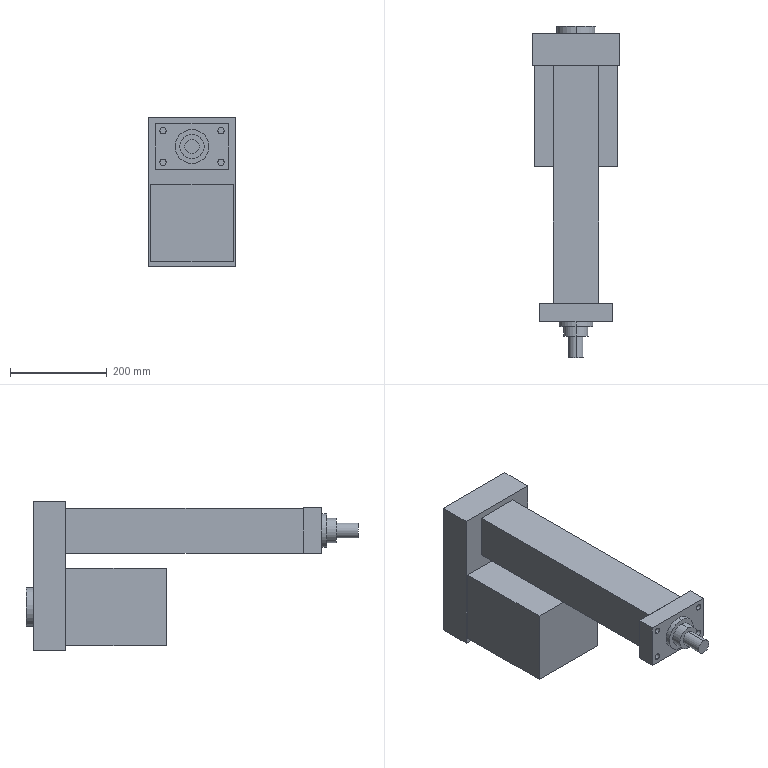Part | STEP file | 1 solid | 41 faces | box 180 x 686 x 308 mm | volume 14325025 mm3 | plane 25 | cylinder 16 | commonest cylinder face diameters 13 x8 30 x2 50 x2 70 x2 80 x2